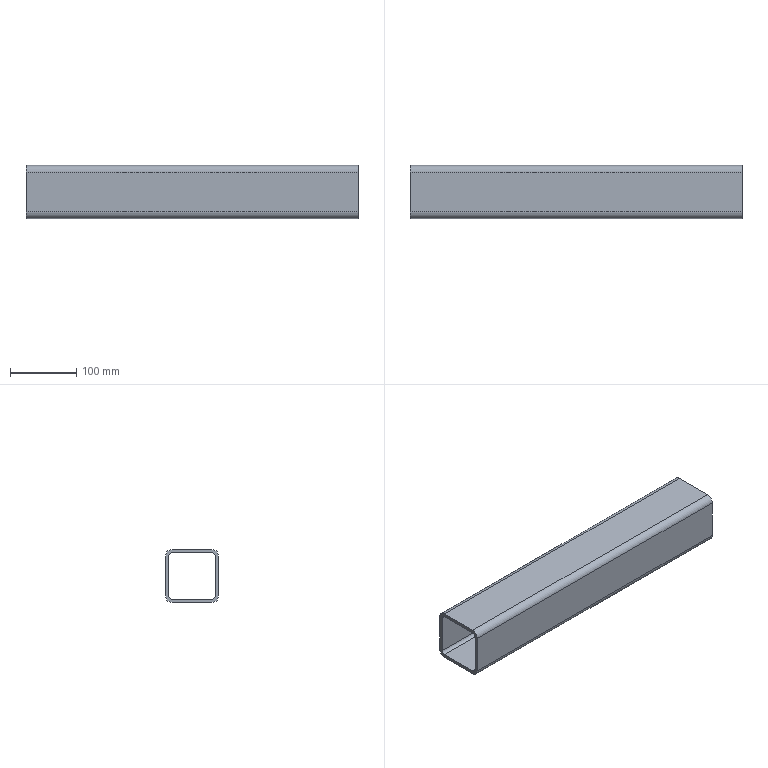Part | SolidWorks | features WeldMemberFeat 1, WeldmentFeature 1 | 1 solid | 18 faces | box 500 x 80 x 80 mm | volume 717810 mm3 | plane 10 | cylinder 8 | commonest cylinder face diameters 10 x4 20 x4
STEP:
#1=CARTESIAN_POINT('',(-250.,30.,-40.));
#2=VERTEX_POINT('',#1);
#3=CARTESIAN_POINT('',(-250.,40.,-30.));
#4=VERTEX_POINT('',#3);
#5=CARTESIAN_POINT('',(-250.,30.,-30.));
#6=DIRECTION('',(1.,0.,0.));
#7=DIRECTION('',(0.,0.,-1.));
#8=AXIS2_PLACEMENT_3D('',#5,#6,#7);
#9=CIRCLE('',#8,10.);
#10=EDGE_CURVE('',#2,#4,#9,.T.);
#11=ORIENTED_EDGE('',*,*,#10,.T.);
#12=CARTESIAN_POINT('',(250.,40.,-30.));
#13=VERTEX_POINT('',#12);
#14=CARTESIAN_POINT('',(250.,40.,-30.));
#15=DIRECTION('',(-1.,0.,0.));
#16=VECTOR('',#15,1000.);
#17=LINE('',#14,#16);
#18=EDGE_CURVE('',#13,#4,#17,.T.);
#19=ORIENTED_EDGE('',*,*,#18,.F.);
#20=CARTESIAN_POINT('',(250.,30.,-40.));
#21=VERTEX_POINT('',#20);
#22=CARTESIAN_POINT('',(250.,30.,-30.));
#23=DIRECTION('',(1.,0.,0.));
#24=DIRECTION('',(0.,0.,-1.));
#25=AXIS2_PLACEMENT_3D('',#22,#23,#24);
#26=CIRCLE('',#25,10.);
#27=EDGE_CURVE('',#21,#13,#26,.T.);
#28=ORIENTED_EDGE('',*,*,#27,.F.);
#29=CARTESIAN_POINT('',(250.,30.,-40.));
#30=DIRECTION('',(-1.,0.,0.));
#31=VECTOR('',#30,1000.);
#32=LINE('',#29,#31);
#33=EDGE_CURVE('',#21,#2,#32,.T.);
#34=ORIENTED_EDGE('',*,*,#33,.T.);
#35=EDGE_LOOP('',(#11,#19,#28,#34));
#36=FACE_OUTER_BOUND('',#35,.T.);
#37=CARTESIAN_POINT('',(250.,30.,-30.));
#38=DIRECTION('',(-1.,0.,0.));
#39=DIRECTION('',(0.,0.,1.));
#40=AXIS2_PLACEMENT_3D('',#37,#38,#39);
#41=CYLINDRICAL_SURFACE('',#40,10.);
#42=ADVANCED_FACE('',(#36),#41,.T.);
#43=CARTESIAN_POINT('',(-250.,40.,30.));
#44=VERTEX_POINT('',#43);
#45=CARTESIAN_POINT('',(-250.,40.,-30.));
#46=DIRECTION('',(0.,0.,1.));
#47=VECTOR('',#46,1000.);
#48=LINE('',#45,#47);
#49=EDGE_CURVE('',#4,#44,#48,.T.);
#50=ORIENTED_EDGE('',*,*,#49,.T.);
#51=CARTESIAN_POINT('',(250.,40.,30.));
#52=VERTEX_POINT('',#51);
#53=CARTESIAN_POINT('',(250.,40.,30.));
#54=DIRECTION('',(-1.,0.,0.));
#55=VECTOR('',#54,1000.);
#56=LINE('',#53,#55);
#57=EDGE_CURVE('',#52,#44,#56,.T.);
#58=ORIENTED_EDGE('',*,*,#57,.F.);
#59=CARTESIAN_POINT('',(250.,40.,-30.));
#60=DIRECTION('',(0.,0.,1.));
#61=VECTOR('',#60,1000.);
#62=LINE('',#59,#61);
#63=EDGE_CURVE('',#13,#52,#62,.T.);
#64=ORIENTED_EDGE('',*,*,#63,.F.);
#65=ORIENTED_EDGE('',*,*,#18,.T.);
#66=EDGE_LOOP('',(#50,#58,#64,#65));
#67=FACE_OUTER_BOUND('',#66,.T.);
#68=CARTESIAN_POINT('',(250.,40.,-30.));
#69=DIRECTION('',(0.,-1.,0.));
#70=DIRECTION('',(0.,0.,-1.));
#71=AXIS2_PLACEMENT_3D('',#68,#69,#70);
#72=PLANE('',#71);
#73=ADVANCED_FACE('',(#67),#72,.F.);
#74=CARTESIAN_POINT('',(-250.,30.,40.));
#75=VERTEX_POINT('',#74);
#76=CARTESIAN_POINT('',(-250.,30.,30.));
#77=DIRECTION('',(1.,0.,0.));
#78=DIRECTION('',(0.,0.,-1.));
#79=AXIS2_PLACEMENT_3D('',#76,#77,#78);
#80=CIRCLE('',#79,10.);
#81=EDGE_CURVE('',#44,#75,#80,.T.);
#82=ORIENTED_EDGE('',*,*,#81,.T.);
#83=CARTESIAN_POINT('',(250.,30.,40.));
#84=VERTEX_POINT('',#83);
#85=CARTESIAN_POINT('',(250.,30.,40.));
#86=DIRECTION('',(-1.,0.,0.));
#87=VECTOR('',#86,1000.);
#88=LINE('',#85,#87);
#89=EDGE_CURVE('',#84,#75,#88,.T.);
#90=ORIENTED_EDGE('',*,*,#89,.F.);
#91=CARTESIAN_POINT('',(250.,30.,30.));
#92=DIRECTION('',(1.,0.,0.));
#93=DIRECTION('',(0.,0.,-1.));
#94=AXIS2_PLACEMENT_3D('',#91,#92,#93);
#95=CIRCLE('',#94,10.);
#96=EDGE_CURVE('',#52,#84,#95,.T.);
#97=ORIENTED_EDGE('',*,*,#96,.F.);
#98=ORIENTED_EDGE('',*,*,#57,.T.);
#99=EDGE_LOOP('',(#82,#90,#97,#98));
#100=FACE_OUTER_BOUND('',#99,.T.);
#101=CARTESIAN_POINT('',(250.,30.,30.));
#102=DIRECTION('',(-1.,0.,0.));
#103=DIRECTION('',(0.,0.,1.));
#104=AXIS2_PLACEMENT_3D('',#101,#102,#103);
#105=CYLINDRICAL_SURFACE('',#104,10.);
#106=ADVANCED_FACE('',(#100),#105,.T.);
#107=CARTESIAN_POINT('',(-250.,-30.,40.));
#108=VERTEX_POINT('',#107);
#109=CARTESIAN_POINT('',(-250.,-30.,40.));
#110=DIRECTION('',(0.,-1.,0.));
#111=VECTOR('',#110,1000.);
#112=LINE('',#109,#111);
#113=EDGE_CURVE('',#75,#108,#112,.T.);
#114=ORIENTED_EDGE('',*,*,#113,.T.);
#115=CARTESIAN_POINT('',(250.,-30.,40.));
#116=VERTEX_POINT('',#115);
#117=CARTESIAN_POINT('',(250.,-30.,40.));
#118=DIRECTION('',(-1.,0.,0.));
#119=VECTOR('',#118,1000.);
#120=LINE('',#117,#119);
#121=EDGE_CURVE('',#116,#108,#120,.T.);
#122=ORIENTED_EDGE('',*,*,#121,.F.);
#123=CARTESIAN_POINT('',(250.,-30.,40.));
#124=DIRECTION('',(0.,-1.,0.));
#125=VECTOR('',#124,1000.);
#126=LINE('',#123,#125);
#127=EDGE_CURVE('',#84,#116,#126,.T.);
#128=ORIENTED_EDGE('',*,*,#127,.F.);
#129=ORIENTED_EDGE('',*,*,#89,.T.);
#130=EDGE_LOOP('',(#114,#122,#128,#129));
#131=FACE_OUTER_BOUND('',#130,.T.);
#132=CARTESIAN_POINT('',(250.,-30.,40.));
#133=DIRECTION('',(0.,0.,-1.));
#134=DIRECTION('',(0.,1.,0.));
#135=AXIS2_PLACEMENT_3D('',#132,#133,#134);
#136=PLANE('',#135);
#137=ADVANCED_FACE('',(#131),#136,.F.);
#138=CARTESIAN_POINT('',(-250.,-40.,30.));
#139=VERTEX_POINT('',#138);
#140=CARTESIAN_POINT('',(-250.,-30.,30.));
#141=DIRECTION('',(1.,0.,0.));
#142=DIRECTION('',(0.,0.,-1.));
#143=AXIS2_PLACEMENT_3D('',#140,#141,#142);
#144=CIRCLE('',#143,10.);
#145=EDGE_CURVE('',#108,#139,#144,.T.);
#146=ORIENTED_EDGE('',*,*,#145,.T.);
#147=CARTESIAN_POINT('',(250.,-40.,30.));
#148=VERTEX_POINT('',#147);
#149=CARTESIAN_POINT('',(250.,-40.,30.));
#150=DIRECTION('',(-1.,0.,0.));
#151=VECTOR('',#150,1000.);
#152=LINE('',#149,#151);
#153=EDGE_CURVE('',#148,#139,#152,.T.);
#154=ORIENTED_EDGE('',*,*,#153,.F.);
#155=CARTESIAN_POINT('',(250.,-30.,30.));
#156=DIRECTION('',(1.,0.,0.));
#157=DIRECTION('',(0.,0.,-1.));
#158=AXIS2_PLACEMENT_3D('',#155,#156,#157);
#159=CIRCLE('',#158,10.);
#160=EDGE_CURVE('',#116,#148,#159,.T.);
#161=ORIENTED_EDGE('',*,*,#160,.F.);
#162=ORIENTED_EDGE('',*,*,#121,.T.);
#163=EDGE_LOOP('',(#146,#154,#161,#162));
#164=FACE_OUTER_BOUND('',#163,.T.);
#165=CARTESIAN_POINT('',(250.,-30.,30.));
#166=DIRECTION('',(-1.,0.,0.));
#167=DIRECTION('',(0.,0.,1.));
#168=AXIS2_PLACEMENT_3D('',#165,#166,#167);
#169=CYLINDRICAL_SURFACE('',#168,10.);
#170=ADVANCED_FACE('',(#164),#169,.T.);
#171=CARTESIAN_POINT('',(-250.,-40.,-30.));
#172=VERTEX_POINT('',#171);
#173=CARTESIAN_POINT('',(-250.,-40.,30.));
#174=DIRECTION('',(0.,0.,-1.));
#175=VECTOR('',#174,1000.);
#176=LINE('',#173,#175);
#177=EDGE_CURVE('',#139,#172,#176,.T.);
#178=ORIENTED_EDGE('',*,*,#177,.T.);
#179=CARTESIAN_POINT('',(250.,-40.,-30.));
#180=VERTEX_POINT('',#179);
#181=CARTESIAN_POINT('',(250.,-40.,-30.));
#182=DIRECTION('',(-1.,0.,0.));
#183=VECTOR('',#182,1000.);
#184=LINE('',#181,#183);
#185=EDGE_CURVE('',#180,#172,#184,.T.);
#186=ORIENTED_EDGE('',*,*,#185,.F.);
#187=CARTESIAN_POINT('',(250.,-40.,30.));
#188=DIRECTION('',(0.,0.,-1.));
#189=VECTOR('',#188,1000.);
#190=LINE('',#187,#189);
#191=EDGE_CURVE('',#148,#180,#190,.T.);
#192=ORIENTED_EDGE('',*,*,#191,.F.);
#193=ORIENTED_EDGE('',*,*,#153,.T.);
#194=EDGE_LOOP('',(#178,#186,#192,#193));
#195=FACE_OUTER_BOUND('',#194,.T.);
#196=CARTESIAN_POINT('',(250.,-40.,30.));
#197=DIRECTION('',(0.,1.,0.));
#198=DIRECTION('',(0.,0.,1.));
#199=AXIS2_PLACEMENT_3D('',#196,#197,#198);
#200=PLANE('',#199);
#201=ADVANCED_FACE('',(#195),#200,.F.);
#202=CARTESIAN_POINT('',(-250.,-30.,-40.));
#203=VERTEX_POINT('',#202);
#204=CARTESIAN_POINT('',(-250.,-30.,-30.));
#205=DIRECTION('',(1.,0.,0.));
#206=DIRECTION('',(0.,0.,-1.));
#207=AXIS2_PLACEMENT_3D('',#204,#205,#206);
#208=CIRCLE('',#207,10.);
#209=EDGE_CURVE('',#172,#203,#208,.T.);
#210=ORIENTED_EDGE('',*,*,#209,.T.);
#211=CARTESIAN_POINT('',(250.,-30.,-40.));
#212=VERTEX_POINT('',#211);
#213=CARTESIAN_POINT('',(250.,-30.,-40.));
#214=DIRECTION('',(-1.,0.,0.));
#215=VECTOR('',#214,1000.);
#216=LINE('',#213,#215);
#217=EDGE_CURVE('',#212,#203,#216,.T.);
#218=ORIENTED_EDGE('',*,*,#217,.F.);
#219=CARTESIAN_POINT('',(250.,-30.,-30.));
#220=DIRECTION('',(1.,0.,0.));
#221=DIRECTION('',(0.,0.,-1.));
#222=AXIS2_PLACEMENT_3D('',#219,#220,#221);
#223=CIRCLE('',#222,10.);
#224=EDGE_CURVE('',#180,#212,#223,.T.);
#225=ORIENTED_EDGE('',*,*,#224,.F.);
#226=ORIENTED_EDGE('',*,*,#185,.T.);
#227=EDGE_LOOP('',(#210,#218,#225,#226));
#228=FACE_OUTER_BOUND('',#227,.T.);
#229=CARTESIAN_POINT('',(250.,-30.,-30.));
#230=DIRECTION('',(-1.,0.,0.));
#231=DIRECTION('',(0.,0.,1.));
#232=AXIS2_PLACEMENT_3D('',#229,#230,#231);
#233=CYLINDRICAL_SURFACE('',#232,10.);
#234=ADVANCED_FACE('',(#228),#233,.T.);
#235=CARTESIAN_POINT('',(-250.,35.,30.));
#236=VERTEX_POINT('',#235);
#237=CARTESIAN_POINT('',(-250.,30.,35.));
#238=VERTEX_POINT('',#237);
#239=CARTESIAN_POINT('',(-250.,30.,30.));
#240=DIRECTION('',(1.,0.,0.));
#241=DIRECTION('',(0.,0.,-1.));
#242=AXIS2_PLACEMENT_3D('',#239,#240,#241);
#243=CIRCLE('',#242,5.);
#244=EDGE_CURVE('',#236,#238,#243,.T.);
#245=ORIENTED_EDGE('',*,*,#244,.F.);
#246=CARTESIAN_POINT('',(250.,35.,30.));
#247=VERTEX_POINT('',#246);
#248=CARTESIAN_POINT('',(250.,35.,30.));
#249=DIRECTION('',(-1.,0.,0.));
#250=VECTOR('',#249,1000.);
#251=LINE('',#248,#250);
#252=EDGE_CURVE('',#247,#236,#251,.T.);
#253=ORIENTED_EDGE('',*,*,#252,.F.);
#254=CARTESIAN_POINT('',(250.,30.,35.));
#255=VERTEX_POINT('',#254);
#256=CARTESIAN_POINT('',(250.,30.,30.));
#257=DIRECTION('',(1.,0.,0.));
#258=DIRECTION('',(0.,0.,-1.));
#259=AXIS2_PLACEMENT_3D('',#256,#257,#258);
#260=CIRCLE('',#259,5.);
#261=EDGE_CURVE('',#247,#255,#260,.T.);
#262=ORIENTED_EDGE('',*,*,#261,.T.);
#263=CARTESIAN_POINT('',(250.,30.,35.));
#264=DIRECTION('',(-1.,0.,0.));
#265=VECTOR('',#264,1000.);
#266=LINE('',#263,#265);
#267=EDGE_CURVE('',#255,#238,#266,.T.);
#268=ORIENTED_EDGE('',*,*,#267,.T.);
#269=EDGE_LOOP('',(#245,#253,#262,#268));
#270=FACE_OUTER_BOUND('',#269,.T.);
#271=CARTESIAN_POINT('',(250.,30.,30.));
#272=DIRECTION('',(-1.,0.,0.));
#273=DIRECTION('',(0.,0.,1.));
#274=AXIS2_PLACEMENT_3D('',#271,#272,#273);
#275=CYLINDRICAL_SURFACE('',#274,5.);
#276=ADVANCED_FACE('',(#270),#275,.F.);
#277=CARTESIAN_POINT('',(-250.,35.,-30.));
#278=VERTEX_POINT('',#277);
#279=CARTESIAN_POINT('',(-250.,35.,-30.));
#280=DIRECTION('',(0.,0.,1.));
#281=VECTOR('',#280,1000.);
#282=LINE('',#279,#281);
#283=EDGE_CURVE('',#278,#236,#282,.T.);
#284=ORIENTED_EDGE('',*,*,#283,.F.);
#285=CARTESIAN_POINT('',(250.,35.,-30.));
#286=VERTEX_POINT('',#285);
#287=CARTESIAN_POINT('',(250.,35.,-30.));
#288=DIRECTION('',(-1.,0.,0.));
#289=VECTOR('',#288,1000.);
#290=LINE('',#287,#289);
#291=EDGE_CURVE('',#286,#278,#290,.T.);
#292=ORIENTED_EDGE('',*,*,#291,.F.);
#293=CARTESIAN_POINT('',(250.,35.,-30.));
#294=DIRECTION('',(0.,0.,1.));
#295=VECTOR('',#294,1000.);
#296=LINE('',#293,#295);
#297=EDGE_CURVE('',#286,#247,#296,.T.);
#298=ORIENTED_EDGE('',*,*,#297,.T.);
#299=ORIENTED_EDGE('',*,*,#252,.T.);
#300=EDGE_LOOP('',(#284,#292,#298,#299));
#301=FACE_OUTER_BOUND('',#300,.T.);
#302=CARTESIAN_POINT('',(250.,35.,-30.));
#303=DIRECTION('',(0.,-1.,0.));
#304=DIRECTION('',(0.,0.,-1.));
#305=AXIS2_PLACEMENT_3D('',#302,#303,#304);
#306=PLANE('',#305);
#307=ADVANCED_FACE('',(#301),#306,.T.);
#308=CARTESIAN_POINT('',(-250.,30.,-35.));
#309=VERTEX_POINT('',#308);
#310=CARTESIAN_POINT('',(-250.,30.,-30.));
#311=DIRECTION('',(1.,0.,0.));
#312=DIRECTION('',(0.,0.,-1.));
#313=AXIS2_PLACEMENT_3D('',#310,#311,#312);
#314=CIRCLE('',#313,5.);
#315=EDGE_CURVE('',#309,#278,#314,.T.);
#316=ORIENTED_EDGE('',*,*,#315,.F.);
#317=CARTESIAN_POINT('',(250.,30.,-35.));
#318=VERTEX_POINT('',#317);
#319=CARTESIAN_POINT('',(250.,30.,-35.));
#320=DIRECTION('',(-1.,0.,0.));
#321=VECTOR('',#320,1000.);
#322=LINE('',#319,#321);
#323=EDGE_CURVE('',#318,#309,#322,.T.);
#324=ORIENTED_EDGE('',*,*,#323,.F.);
#325=CARTESIAN_POINT('',(250.,30.,-30.));
#326=DIRECTION('',(1.,0.,0.));
#327=DIRECTION('',(0.,0.,-1.));
#328=AXIS2_PLACEMENT_3D('',#325,#326,#327);
#329=CIRCLE('',#328,5.);
#330=EDGE_CURVE('',#318,#286,#329,.T.);
#331=ORIENTED_EDGE('',*,*,#330,.T.);
#332=ORIENTED_EDGE('',*,*,#291,.T.);
#333=EDGE_LOOP('',(#316,#324,#331,#332));
#334=FACE_OUTER_BOUND('',#333,.T.);
#335=CARTESIAN_POINT('',(250.,30.,-30.));
#336=DIRECTION('',(-1.,0.,0.));
#337=DIRECTION('',(0.,0.,1.));
#338=AXIS2_PLACEMENT_3D('',#335,#336,#337);
#339=CYLINDRICAL_SURFACE('',#338,5.);
#340=ADVANCED_FACE('',(#334),#339,.F.);
#341=CARTESIAN_POINT('',(-250.,-30.,-35.));
#342=VERTEX_POINT('',#341);
#343=CARTESIAN_POINT('',(-250.,30.,-35.));
#344=DIRECTION('',(0.,1.,0.));
#345=VECTOR('',#344,1000.);
#346=LINE('',#343,#345);
#347=EDGE_CURVE('',#342,#309,#346,.T.);
#348=ORIENTED_EDGE('',*,*,#347,.F.);
#349=CARTESIAN_POINT('',(250.,-30.,-35.));
#350=VERTEX_POINT('',#349);
#351=CARTESIAN_POINT('',(250.,-30.,-35.));
#352=DIRECTION('',(-1.,0.,0.));
#353=VECTOR('',#352,1000.);
#354=LINE('',#351,#353);
#355=EDGE_CURVE('',#350,#342,#354,.T.);
#356=ORIENTED_EDGE('',*,*,#355,.F.);
#357=CARTESIAN_POINT('',(250.,30.,-35.));
#358=DIRECTION('',(0.,1.,0.));
#359=VECTOR('',#358,1000.);
#360=LINE('',#357,#359);
#361=EDGE_CURVE('',#350,#318,#360,.T.);
#362=ORIENTED_EDGE('',*,*,#361,.T.);
#363=ORIENTED_EDGE('',*,*,#323,.T.);
#364=EDGE_LOOP('',(#348,#356,#362,#363));
#365=FACE_OUTER_BOUND('',#364,.T.);
#366=CARTESIAN_POINT('',(250.,30.,-35.));
#367=DIRECTION('',(0.,0.,1.));
#368=DIRECTION('',(1.,0.,0.));
#369=AXIS2_PLACEMENT_3D('',#366,#367,#368);
#370=PLANE('',#369);
#371=ADVANCED_FACE('',(#365),#370,.T.);
#372=CARTESIAN_POINT('',(-250.,-35.,-30.));
#373=VERTEX_POINT('',#372);
#374=CARTESIAN_POINT('',(-250.,-30.,-30.));
#375=DIRECTION('',(1.,0.,0.));
#376=DIRECTION('',(0.,0.,-1.));
#377=AXIS2_PLACEMENT_3D('',#374,#375,#376);
#378=CIRCLE('',#377,5.);
#379=EDGE_CURVE('',#373,#342,#378,.T.);
#380=ORIENTED_EDGE('',*,*,#379,.F.);
#381=CARTESIAN_POINT('',(250.,-35.,-30.));
#382=VERTEX_POINT('',#381);
#383=CARTESIAN_POINT('',(250.,-35.,-30.));
#384=DIRECTION('',(-1.,0.,0.));
#385=VECTOR('',#384,1000.);
#386=LINE('',#383,#385);
#387=EDGE_CURVE('',#382,#373,#386,.T.);
#388=ORIENTED_EDGE('',*,*,#387,.F.);
#389=CARTESIAN_POINT('',(250.,-30.,-30.));
#390=DIRECTION('',(1.,0.,0.));
#391=DIRECTION('',(0.,0.,-1.));
#392=AXIS2_PLACEMENT_3D('',#389,#390,#391);
#393=CIRCLE('',#392,5.);
#394=EDGE_CURVE('',#382,#350,#393,.T.);
#395=ORIENTED_EDGE('',*,*,#394,.T.);
#396=ORIENTED_EDGE('',*,*,#355,.T.);
#397=EDGE_LOOP('',(#380,#388,#395,#396));
#398=FACE_OUTER_BOUND('',#397,.T.);
#399=CARTESIAN_POINT('',(250.,-30.,-30.));
#400=DIRECTION('',(-1.,0.,0.));
#401=DIRECTION('',(0.,0.,1.));
#402=AXIS2_PLACEMENT_3D('',#399,#400,#401);
#403=CYLINDRICAL_SURFACE('',#402,5.);
#404=ADVANCED_FACE('',(#398),#403,.F.);
#405=CARTESIAN_POINT('',(-250.,-35.,30.));
#406=VERTEX_POINT('',#405);
#407=CARTESIAN_POINT('',(-250.,-35.,30.));
#408=DIRECTION('',(0.,0.,-1.));
#409=VECTOR('',#408,1000.);
#410=LINE('',#407,#409);
#411=EDGE_CURVE('',#406,#373,#410,.T.);
#412=ORIENTED_EDGE('',*,*,#411,.F.);
#413=CARTESIAN_POINT('',(250.,-35.,30.));
#414=VERTEX_POINT('',#413);
#415=CARTESIAN_POINT('',(250.,-35.,30.));
#416=DIRECTION('',(-1.,0.,0.));
#417=VECTOR('',#416,1000.);
#418=LINE('',#415,#417);
#419=EDGE_CURVE('',#414,#406,#418,.T.);
#420=ORIENTED_EDGE('',*,*,#419,.F.);
#421=CARTESIAN_POINT('',(250.,-35.,30.));
#422=DIRECTION('',(0.,0.,-1.));
#423=VECTOR('',#422,1000.);
#424=LINE('',#421,#423);
#425=EDGE_CURVE('',#414,#382,#424,.T.);
#426=ORIENTED_EDGE('',*,*,#425,.T.);
#427=ORIENTED_EDGE('',*,*,#387,.T.);
#428=EDGE_LOOP('',(#412,#420,#426,#427));
#429=FACE_OUTER_BOUND('',#428,.T.);
#430=CARTESIAN_POINT('',(250.,-35.,30.));
#431=DIRECTION('',(0.,1.,0.));
#432=DIRECTION('',(0.,0.,1.));
#433=AXIS2_PLACEMENT_3D('',#430,#431,#432);
#434=PLANE('',#433);
#435=ADVANCED_FACE('',(#429),#434,.T.);
#436=CARTESIAN_POINT('',(-250.,-30.,35.));
#437=VERTEX_POINT('',#436);
#438=CARTESIAN_POINT('',(-250.,-30.,30.));
#439=DIRECTION('',(1.,0.,0.));
#440=DIRECTION('',(0.,0.,-1.));
#441=AXIS2_PLACEMENT_3D('',#438,#439,#440);
#442=CIRCLE('',#441,5.);
#443=EDGE_CURVE('',#437,#406,#442,.T.);
#444=ORIENTED_EDGE('',*,*,#443,.F.);
#445=CARTESIAN_POINT('',(250.,-30.,35.));
#446=VERTEX_POINT('',#445);
#447=CARTESIAN_POINT('',(250.,-30.,35.));
#448=DIRECTION('',(-1.,0.,0.));
#449=VECTOR('',#448,1000.);
#450=LINE('',#447,#449);
#451=EDGE_CURVE('',#446,#437,#450,.T.);
#452=ORIENTED_EDGE('',*,*,#451,.F.);
#453=CARTESIAN_POINT('',(250.,-30.,30.));
#454=DIRECTION('',(1.,0.,0.));
#455=DIRECTION('',(0.,0.,-1.));
#456=AXIS2_PLACEMENT_3D('',#453,#454,#455);
#457=CIRCLE('',#456,5.);
#458=EDGE_CURVE('',#446,#414,#457,.T.);
#459=ORIENTED_EDGE('',*,*,#458,.T.);
#460=ORIENTED_EDGE('',*,*,#419,.T.);
#461=EDGE_LOOP('',(#444,#452,#459,#460));
#462=FACE_OUTER_BOUND('',#461,.T.);
#463=CARTESIAN_POINT('',(250.,-30.,30.));
#464=DIRECTION('',(-1.,0.,0.));
#465=DIRECTION('',(0.,0.,1.));
#466=AXIS2_PLACEMENT_3D('',#463,#464,#465);
#467=CYLINDRICAL_SURFACE('',#466,5.);
#468=ADVANCED_FACE('',(#462),#467,.F.);
#469=CARTESIAN_POINT('',(-250.,-30.,35.));
#470=DIRECTION('',(0.,-1.,0.));
#471=VECTOR('',#470,1000.);
#472=LINE('',#469,#471);
#473=EDGE_CURVE('',#238,#437,#472,.T.);
#474=ORIENTED_EDGE('',*,*,#473,.F.);
#475=ORIENTED_EDGE('',*,*,#267,.F.);
#476=CARTESIAN_POINT('',(250.,-30.,35.));
#477=DIRECTION('',(0.,-1.,0.));
#478=VECTOR('',#477,1000.);
#479=LINE('',#476,#478);
#480=EDGE_CURVE('',#255,#446,#479,.T.);
#481=ORIENTED_EDGE('',*,*,#480,.T.);
#482=ORIENTED_EDGE('',*,*,#451,.T.);
#483=EDGE_LOOP('',(#474,#475,#481,#482));
#484=FACE_OUTER_BOUND('',#483,.T.);
#485=CARTESIAN_POINT('',(250.,-30.,35.));
#486=DIRECTION('',(0.,0.,-1.));
#487=DIRECTION('',(0.,1.,0.));
#488=AXIS2_PLACEMENT_3D('',#485,#486,#487);
#489=PLANE('',#488);
#490=ADVANCED_FACE('',(#484),#489,.T.);
#491=CARTESIAN_POINT('',(-250.,30.,-40.));
#492=DIRECTION('',(0.,1.,0.));
#493=VECTOR('',#492,1000.);
#494=LINE('',#491,#493);
#495=EDGE_CURVE('',#203,#2,#494,.T.);
#496=ORIENTED_EDGE('',*,*,#495,.T.);
#497=ORIENTED_EDGE('',*,*,#33,.F.);
#498=CARTESIAN_POINT('',(250.,30.,-40.));
#499=DIRECTION('',(0.,1.,0.));
#500=VECTOR('',#499,1000.);
#501=LINE('',#498,#500);
#502=EDGE_CURVE('',#212,#21,#501,.T.);
#503=ORIENTED_EDGE('',*,*,#502,.F.);
#504=ORIENTED_EDGE('',*,*,#217,.T.);
#505=EDGE_LOOP('',(#496,#497,#503,#504));
#506=FACE_OUTER_BOUND('',#505,.T.);
#507=CARTESIAN_POINT('',(250.,30.,-40.));
#508=DIRECTION('',(0.,0.,1.));
#509=DIRECTION('',(1.,0.,0.));
#510=AXIS2_PLACEMENT_3D('',#507,#508,#509);
#511=PLANE('',#510);
#512=ADVANCED_FACE('',(#506),#511,.F.);
#513=ORIENTED_EDGE('',*,*,#261,.F.);
#514=ORIENTED_EDGE('',*,*,#297,.F.);
#515=ORIENTED_EDGE('',*,*,#330,.F.);
#516=ORIENTED_EDGE('',*,*,#361,.F.);
#517=ORIENTED_EDGE('',*,*,#394,.F.);
#518=ORIENTED_EDGE('',*,*,#425,.F.);
#519=ORIENTED_EDGE('',*,*,#458,.F.);
#520=ORIENTED_EDGE('',*,*,#480,.F.);
#521=EDGE_LOOP('',(#513,#514,#515,#516,#517,#518,#519,#520));
#522=FACE_BOUND('',#521,.T.);
#523=ORIENTED_EDGE('',*,*,#27,.T.);
#524=ORIENTED_EDGE('',*,*,#63,.T.);
#525=ORIENTED_EDGE('',*,*,#96,.T.);
#526=ORIENTED_EDGE('',*,*,#127,.T.);
#527=ORIENTED_EDGE('',*,*,#160,.T.);
#528=ORIENTED_EDGE('',*,*,#191,.T.);
#529=ORIENTED_EDGE('',*,*,#224,.T.);
#530=ORIENTED_EDGE('',*,*,#502,.T.);
#531=EDGE_LOOP('',(#523,#524,#525,#526,#527,#528,#529,#530));
#532=FACE_OUTER_BOUND('',#531,.T.);
#533=CARTESIAN_POINT('',(250.,30.,-30.));
#534=DIRECTION('',(1.,0.,0.));
#535=DIRECTION('',(0.,0.,-1.));
#536=AXIS2_PLACEMENT_3D('',#533,#534,#535);
#537=PLANE('',#536);
#538=ADVANCED_FACE('',(#522,#532),#537,.T.);
#539=ORIENTED_EDGE('',*,*,#244,.T.);
#540=ORIENTED_EDGE('',*,*,#473,.T.);
#541=ORIENTED_EDGE('',*,*,#443,.T.);
#542=ORIENTED_EDGE('',*,*,#411,.T.);
#543=ORIENTED_EDGE('',*,*,#379,.T.);
#544=ORIENTED_EDGE('',*,*,#347,.T.);
#545=ORIENTED_EDGE('',*,*,#315,.T.);
#546=ORIENTED_EDGE('',*,*,#283,.T.);
#547=EDGE_LOOP('',(#539,#540,#541,#542,#543,#544,#545,#546));
#548=FACE_BOUND('',#547,.T.);
#549=ORIENTED_EDGE('',*,*,#10,.F.);
#550=ORIENTED_EDGE('',*,*,#495,.F.);
#551=ORIENTED_EDGE('',*,*,#209,.F.);
#552=ORIENTED_EDGE('',*,*,#177,.F.);
#553=ORIENTED_EDGE('',*,*,#145,.F.);
#554=ORIENTED_EDGE('',*,*,#113,.F.);
#555=ORIENTED_EDGE('',*,*,#81,.F.);
#556=ORIENTED_EDGE('',*,*,#49,.F.);
#557=EDGE_LOOP('',(#549,#550,#551,#552,#553,#554,#555,#556));
#558=FACE_OUTER_BOUND('',#557,.T.);
#559=CARTESIAN_POINT('',(-250.,30.,-30.));
#560=DIRECTION('',(1.,0.,0.));
#561=DIRECTION('',(0.,0.,-1.));
#562=AXIS2_PLACEMENT_3D('',#559,#560,#561);
#563=PLANE('',#562);
#564=ADVANCED_FACE('',(#548,#558),#563,.F.);
#565=CLOSED_SHELL('',(#42,#73,#106,#137,#170,#201,#234,#276,#307,#340,#371,#404,#435,#468,#490,#512,#538,#564));
#566=MANIFOLD_SOLID_BREP('',#565);
#567=CARTESIAN_POINT('',(0.,0.,0.));
#568=DIRECTION('',(0.,0.,1.));
#569=DIRECTION('',(1.,0.,0.));
#570=AXIS2_PLACEMENT_3D('',#567,#568,#569);
#571=(LENGTH_UNIT()NAMED_UNIT(*)SI_UNIT(.MILLI.,.METRE.));
#572=UNCERTAINTY_MEASURE_WITH_UNIT(LENGTH_MEASURE(0.00001),#571,'','');
#573=(NAMED_UNIT(*)PLANE_ANGLE_UNIT()SI_UNIT($,.RADIAN.));
#574=(NAMED_UNIT(*)SI_UNIT($,.STERADIAN.)SOLID_ANGLE_UNIT());
#575=(GEOMETRIC_REPRESENTATION_CONTEXT(3)GLOBAL_UNCERTAINTY_ASSIGNED_CONTEXT((#572))GLOBAL_UNIT_ASSIGNED_CONTEXT((#571,#573,#574))REPRESENTATION_CONTEXT('',''));
#576=ADVANCED_BREP_SHAPE_REPRESENTATION('',(#566,#570),#575);